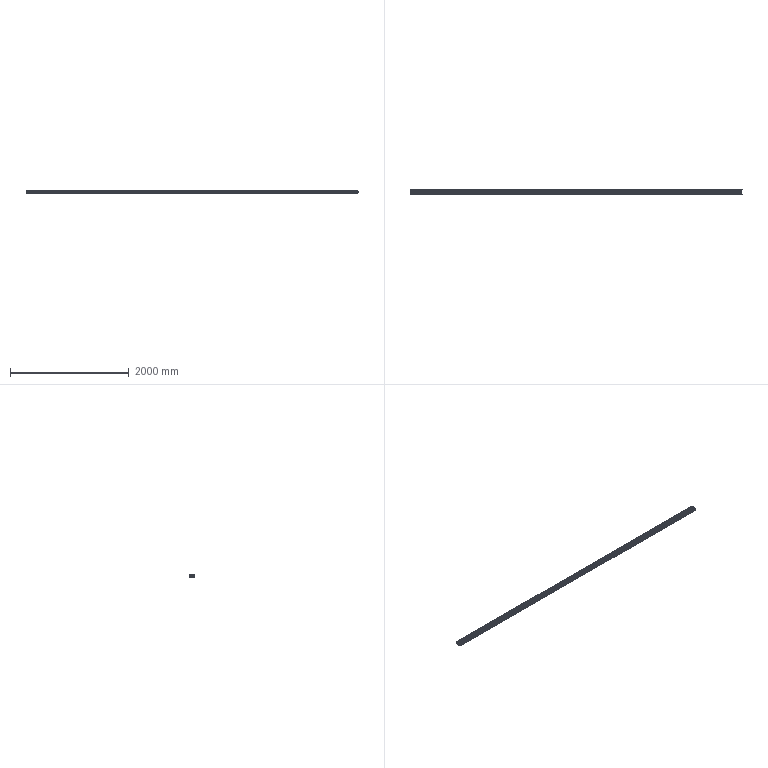Part | STEP file | 1 | 1 solid | 128 faces | box 5600 x 90 x 45 mm | volume 9330158 mm3 | plane 102 | cylinder 26 | commonest cylinder face diameters 2 x16 6 x4 8 x4 10 x2